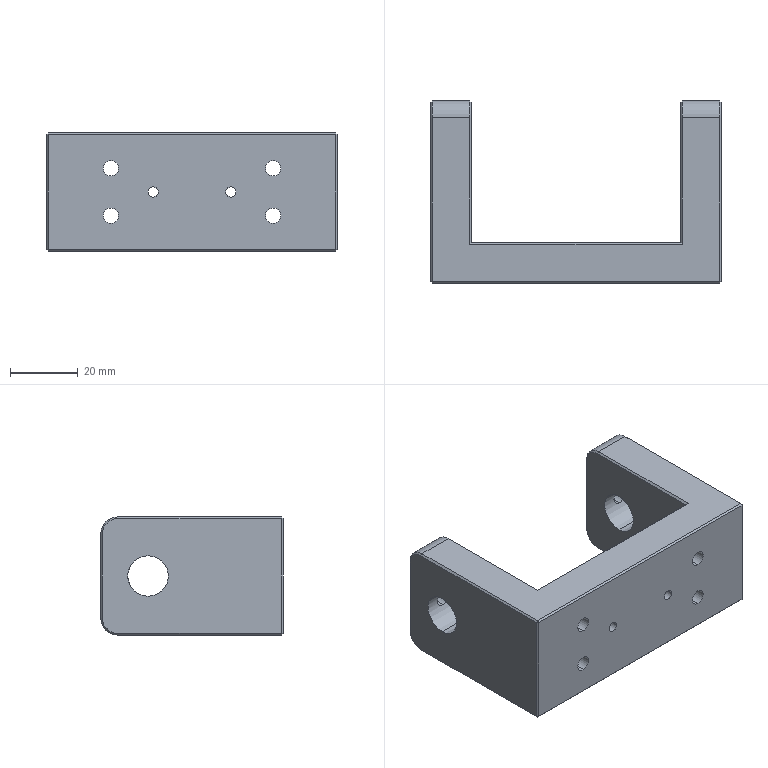Part | STEP file | ND25021-01-JDKM-61-TL | 1 solid | 76 faces | box 86 x 54 x 35 mm | volume 66557 mm3 | plane 36 | cylinder 32 | cone 8 | commonest cylinder face diameters 4.5 x8 8 x8 3 x4 4.2 x4 10 x4 12 x4